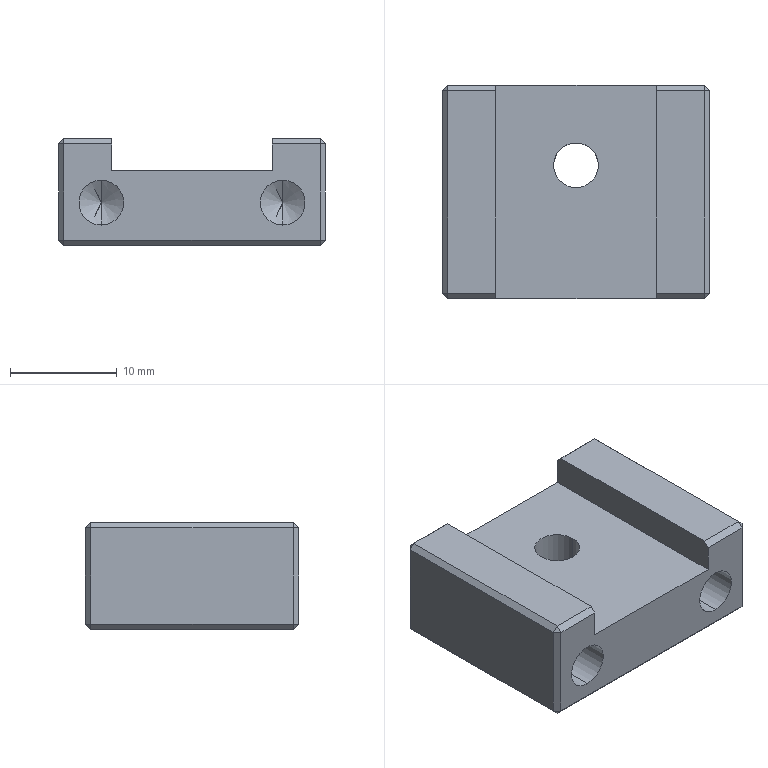Part | SolidWorks | features HoleWzd 2, Chamfer 1, Extrusion 1, ICE 1 | 1 solid | 42 faces | box 25 x 20 x 10 mm | volume 3625 mm3 | plane 32 | cylinder 6 | cone 4 | commonest cylinder face diameters 4.2 x6
STEP:
#1=CARTESIAN_POINT('',(-8.5,2.4,6.1));
#2=VERTEX_POINT('',#1);
#3=CARTESIAN_POINT('',(-8.5,2.4,1.9));
#4=VERTEX_POINT('',#3);
#5=CARTESIAN_POINT('',(-8.5,2.4,4.));
#6=DIRECTION('',(0.,-1.,0.));
#7=DIRECTION('',(0.,0.,-1.));
#8=AXIS2_PLACEMENT_3D('',#5,#6,#7);
#9=CIRCLE('',#8,2.1);
#10=EDGE_CURVE('',#2,#4,#9,.T.);
#11=ORIENTED_EDGE('',*,*,#10,.F.);
#12=CARTESIAN_POINT('',(-8.5,-10.,6.1));
#13=VERTEX_POINT('',#12);
#14=CARTESIAN_POINT('',(-8.5,-10.,6.1));
#15=DIRECTION('',(0.,-1.,0.));
#16=VECTOR('',#15,1000.);
#17=LINE('',#14,#16);
#18=EDGE_CURVE('',#2,#13,#17,.T.);
#19=ORIENTED_EDGE('',*,*,#18,.T.);
#20=CARTESIAN_POINT('',(-8.5,-10.,1.9));
#21=VERTEX_POINT('',#20);
#22=CARTESIAN_POINT('',(-8.5,-10.,4.));
#23=DIRECTION('',(0.,-1.,0.));
#24=DIRECTION('',(0.,0.,-1.));
#25=AXIS2_PLACEMENT_3D('',#22,#23,#24);
#26=CIRCLE('',#25,2.1);
#27=EDGE_CURVE('',#13,#21,#26,.T.);
#28=ORIENTED_EDGE('',*,*,#27,.T.);
#29=CARTESIAN_POINT('',(-8.5,-10.,1.9));
#30=DIRECTION('',(0.,-1.,0.));
#31=VECTOR('',#30,1000.);
#32=LINE('',#29,#31);
#33=EDGE_CURVE('',#4,#21,#32,.T.);
#34=ORIENTED_EDGE('',*,*,#33,.F.);
#35=EDGE_LOOP('',(#11,#19,#28,#34));
#36=FACE_OUTER_BOUND('',#35,.T.);
#37=CARTESIAN_POINT('',(-8.5,-10.,4.));
#38=DIRECTION('',(0.,-1.,0.));
#39=DIRECTION('',(0.,0.,-1.));
#40=AXIS2_PLACEMENT_3D('',#37,#38,#39);
#41=CYLINDRICAL_SURFACE('',#40,2.1);
#42=ADVANCED_FACE('',(#36),#41,.F.);
#43=CARTESIAN_POINT('',(-8.5,3.662,4.));
#44=VERTEX_POINT('',#43);
#45=CARTESIAN_POINT('',(-8.5,2.4,1.9));
#46=DIRECTION('',(0.,-0.515,-0.8572));
#47=VECTOR('',#46,1000.);
#48=LINE('',#45,#47);
#49=EDGE_CURVE('',#44,#4,#48,.T.);
#50=ORIENTED_EDGE('',*,*,#49,.F.);
#51=CARTESIAN_POINT('',(-8.5,2.4,6.1));
#52=DIRECTION('',(0.,-0.515,0.8572));
#53=VECTOR('',#52,1000.);
#54=LINE('',#51,#53);
#55=EDGE_CURVE('',#44,#2,#54,.T.);
#56=ORIENTED_EDGE('',*,*,#55,.T.);
#57=ORIENTED_EDGE('',*,*,#10,.T.);
#58=EDGE_LOOP('',(#50,#56,#57));
#59=FACE_OUTER_BOUND('',#58,.T.);
#60=CARTESIAN_POINT('',(-8.5,2.4,4.));
#61=DIRECTION('',(0.,-1.,0.));
#62=DIRECTION('',(0.,0.,-1.));
#63=AXIS2_PLACEMENT_3D('',#60,#61,#62);
#64=CONICAL_SURFACE('',#63,2.1,1.03);
#65=ADVANCED_FACE('',(#59),#64,.F.);
#66=CARTESIAN_POINT('',(8.5,2.4,6.1));
#67=VERTEX_POINT('',#66);
#68=CARTESIAN_POINT('',(8.5,2.4,1.9));
#69=VERTEX_POINT('',#68);
#70=CARTESIAN_POINT('',(8.5,2.4,4.));
#71=DIRECTION('',(0.,-1.,0.));
#72=DIRECTION('',(0.,0.,-1.));
#73=AXIS2_PLACEMENT_3D('',#70,#71,#72);
#74=CIRCLE('',#73,2.1);
#75=EDGE_CURVE('',#67,#69,#74,.T.);
#76=ORIENTED_EDGE('',*,*,#75,.F.);
#77=CARTESIAN_POINT('',(8.5,-10.,6.1));
#78=VERTEX_POINT('',#77);
#79=CARTESIAN_POINT('',(8.5,-10.,6.1));
#80=DIRECTION('',(0.,-1.,0.));
#81=VECTOR('',#80,1000.);
#82=LINE('',#79,#81);
#83=EDGE_CURVE('',#67,#78,#82,.T.);
#84=ORIENTED_EDGE('',*,*,#83,.T.);
#85=CARTESIAN_POINT('',(8.5,-10.,1.9));
#86=VERTEX_POINT('',#85);
#87=CARTESIAN_POINT('',(8.5,-10.,4.));
#88=DIRECTION('',(0.,-1.,0.));
#89=DIRECTION('',(0.,0.,-1.));
#90=AXIS2_PLACEMENT_3D('',#87,#88,#89);
#91=CIRCLE('',#90,2.1);
#92=EDGE_CURVE('',#78,#86,#91,.T.);
#93=ORIENTED_EDGE('',*,*,#92,.T.);
#94=CARTESIAN_POINT('',(8.5,-10.,1.9));
#95=DIRECTION('',(0.,-1.,0.));
#96=VECTOR('',#95,1000.);
#97=LINE('',#94,#96);
#98=EDGE_CURVE('',#69,#86,#97,.T.);
#99=ORIENTED_EDGE('',*,*,#98,.F.);
#100=EDGE_LOOP('',(#76,#84,#93,#99));
#101=FACE_OUTER_BOUND('',#100,.T.);
#102=CARTESIAN_POINT('',(8.5,-10.,4.));
#103=DIRECTION('',(0.,-1.,0.));
#104=DIRECTION('',(0.,0.,-1.));
#105=AXIS2_PLACEMENT_3D('',#102,#103,#104);
#106=CYLINDRICAL_SURFACE('',#105,2.1);
#107=ADVANCED_FACE('',(#101),#106,.F.);
#108=CARTESIAN_POINT('',(8.5,3.662,4.));
#109=VERTEX_POINT('',#108);
#110=CARTESIAN_POINT('',(8.5,2.4,1.9));
#111=DIRECTION('',(0.,-0.515,-0.8572));
#112=VECTOR('',#111,1000.);
#113=LINE('',#110,#112);
#114=EDGE_CURVE('',#109,#69,#113,.T.);
#115=ORIENTED_EDGE('',*,*,#114,.F.);
#116=CARTESIAN_POINT('',(8.5,2.4,6.1));
#117=DIRECTION('',(0.,-0.515,0.8572));
#118=VECTOR('',#117,1000.);
#119=LINE('',#116,#118);
#120=EDGE_CURVE('',#109,#67,#119,.T.);
#121=ORIENTED_EDGE('',*,*,#120,.T.);
#122=ORIENTED_EDGE('',*,*,#75,.T.);
#123=EDGE_LOOP('',(#115,#121,#122));
#124=FACE_OUTER_BOUND('',#123,.T.);
#125=CARTESIAN_POINT('',(8.5,2.4,4.));
#126=DIRECTION('',(0.,-1.,0.));
#127=DIRECTION('',(0.,0.,-1.));
#128=AXIS2_PLACEMENT_3D('',#125,#126,#127);
#129=CONICAL_SURFACE('',#128,2.1,1.03);
#130=ADVANCED_FACE('',(#124),#129,.F.);
#131=CARTESIAN_POINT('',(-2.1,2.5,0.));
#132=VERTEX_POINT('',#131);
#133=CARTESIAN_POINT('',(2.1,2.5,0.));
#134=VERTEX_POINT('',#133);
#135=CARTESIAN_POINT('',(0.,2.5,0.));
#136=DIRECTION('',(0.,0.,1.));
#137=DIRECTION('',(1.,0.,0.));
#138=AXIS2_PLACEMENT_3D('',#135,#136,#137);
#139=CIRCLE('',#138,2.1);
#140=EDGE_CURVE('',#132,#134,#139,.T.);
#141=ORIENTED_EDGE('',*,*,#140,.F.);
#142=CARTESIAN_POINT('',(-2.1,2.5,7.));
#143=VERTEX_POINT('',#142);
#144=CARTESIAN_POINT('',(-2.1,2.5,7.));
#145=DIRECTION('',(0.,0.,1.));
#146=VECTOR('',#145,1000.);
#147=LINE('',#144,#146);
#148=EDGE_CURVE('',#132,#143,#147,.T.);
#149=ORIENTED_EDGE('',*,*,#148,.T.);
#150=CARTESIAN_POINT('',(2.1,2.5,7.));
#151=VERTEX_POINT('',#150);
#152=CARTESIAN_POINT('',(0.,2.5,7.));
#153=DIRECTION('',(0.,0.,1.));
#154=DIRECTION('',(1.,0.,0.));
#155=AXIS2_PLACEMENT_3D('',#152,#153,#154);
#156=CIRCLE('',#155,2.1);
#157=EDGE_CURVE('',#143,#151,#156,.T.);
#158=ORIENTED_EDGE('',*,*,#157,.T.);
#159=CARTESIAN_POINT('',(2.1,2.5,7.));
#160=DIRECTION('',(0.,0.,1.));
#161=VECTOR('',#160,1000.);
#162=LINE('',#159,#161);
#163=EDGE_CURVE('',#134,#151,#162,.T.);
#164=ORIENTED_EDGE('',*,*,#163,.F.);
#165=EDGE_LOOP('',(#141,#149,#158,#164));
#166=FACE_OUTER_BOUND('',#165,.T.);
#167=CARTESIAN_POINT('',(0.,2.5,7.));
#168=DIRECTION('',(0.,0.,1.));
#169=DIRECTION('',(1.,0.,0.));
#170=AXIS2_PLACEMENT_3D('',#167,#168,#169);
#171=CYLINDRICAL_SURFACE('',#170,2.1);
#172=ADVANCED_FACE('',(#166),#171,.F.);
#173=CARTESIAN_POINT('',(12.,-10.,0.5));
#174=VERTEX_POINT('',#173);
#175=CARTESIAN_POINT('',(12.,-10.,9.5));
#176=VERTEX_POINT('',#175);
#177=CARTESIAN_POINT('',(12.,-10.,10.));
#178=DIRECTION('',(0.,0.,1.));
#179=VECTOR('',#178,1000.);
#180=LINE('',#177,#179);
#181=EDGE_CURVE('',#174,#176,#180,.T.);
#182=ORIENTED_EDGE('',*,*,#181,.T.);
#183=CARTESIAN_POINT('',(7.5,-10.,9.5));
#184=VERTEX_POINT('',#183);
#185=CARTESIAN_POINT('',(-12.5,-10.,9.5));
#186=DIRECTION('',(-1.,0.,0.));
#187=VECTOR('',#186,1000.);
#188=LINE('',#185,#187);
#189=EDGE_CURVE('',#176,#184,#188,.T.);
#190=ORIENTED_EDGE('',*,*,#189,.T.);
#191=CARTESIAN_POINT('',(7.5,-10.,7.));
#192=VERTEX_POINT('',#191);
#193=CARTESIAN_POINT('',(7.5,-10.,7.));
#194=DIRECTION('',(0.,0.,1.));
#195=VECTOR('',#194,1000.);
#196=LINE('',#193,#195);
#197=EDGE_CURVE('',#192,#184,#196,.T.);
#198=ORIENTED_EDGE('',*,*,#197,.F.);
#199=CARTESIAN_POINT('',(-7.5,-10.,7.));
#200=VERTEX_POINT('',#199);
#201=CARTESIAN_POINT('',(-7.5,-10.,7.));
#202=DIRECTION('',(1.,0.,0.));
#203=VECTOR('',#202,1000.);
#204=LINE('',#201,#203);
#205=EDGE_CURVE('',#200,#192,#204,.T.);
#206=ORIENTED_EDGE('',*,*,#205,.F.);
#207=CARTESIAN_POINT('',(-7.5,-10.,9.5));
#208=VERTEX_POINT('',#207);
#209=CARTESIAN_POINT('',(-7.5,-10.,7.));
#210=DIRECTION('',(0.,0.,1.));
#211=VECTOR('',#210,1000.);
#212=LINE('',#209,#211);
#213=EDGE_CURVE('',#200,#208,#212,.T.);
#214=ORIENTED_EDGE('',*,*,#213,.T.);
#215=CARTESIAN_POINT('',(-12.,-10.,9.5));
#216=VERTEX_POINT('',#215);
#217=CARTESIAN_POINT('',(-12.5,-10.,9.5));
#218=DIRECTION('',(-1.,0.,0.));
#219=VECTOR('',#218,1000.);
#220=LINE('',#217,#219);
#221=EDGE_CURVE('',#208,#216,#220,.T.);
#222=ORIENTED_EDGE('',*,*,#221,.T.);
#223=CARTESIAN_POINT('',(-12.,-10.,0.5));
#224=VERTEX_POINT('',#223);
#225=CARTESIAN_POINT('',(-12.,-10.,10.));
#226=DIRECTION('',(0.,0.,-1.));
#227=VECTOR('',#226,1000.);
#228=LINE('',#225,#227);
#229=EDGE_CURVE('',#216,#224,#228,.T.);
#230=ORIENTED_EDGE('',*,*,#229,.T.);
#231=CARTESIAN_POINT('',(12.5,-10.,0.5));
#232=DIRECTION('',(1.,0.,0.));
#233=VECTOR('',#232,1000.);
#234=LINE('',#231,#233);
#235=EDGE_CURVE('',#224,#174,#234,.T.);
#236=ORIENTED_EDGE('',*,*,#235,.T.);
#237=EDGE_LOOP('',(#182,#190,#198,#206,#214,#222,#230,#236));
#238=FACE_OUTER_BOUND('',#237,.T.);
#239=CARTESIAN_POINT('',(8.5,-10.,4.));
#240=DIRECTION('',(0.,-1.,0.));
#241=DIRECTION('',(0.,0.,-1.));
#242=AXIS2_PLACEMENT_3D('',#239,#240,#241);
#243=CIRCLE('',#242,2.1);
#244=EDGE_CURVE('',#86,#78,#243,.T.);
#245=ORIENTED_EDGE('',*,*,#244,.F.);
#246=ORIENTED_EDGE('',*,*,#92,.F.);
#247=EDGE_LOOP('',(#245,#246));
#248=FACE_BOUND('',#247,.T.);
#249=CARTESIAN_POINT('',(-8.5,-10.,4.));
#250=DIRECTION('',(0.,-1.,0.));
#251=DIRECTION('',(0.,0.,-1.));
#252=AXIS2_PLACEMENT_3D('',#249,#250,#251);
#253=CIRCLE('',#252,2.1);
#254=EDGE_CURVE('',#21,#13,#253,.T.);
#255=ORIENTED_EDGE('',*,*,#254,.F.);
#256=ORIENTED_EDGE('',*,*,#27,.F.);
#257=EDGE_LOOP('',(#255,#256));
#258=FACE_BOUND('',#257,.T.);
#259=CARTESIAN_POINT('',(-12.5,-10.,10.));
#260=DIRECTION('',(0.,1.,0.));
#261=DIRECTION('',(0.,0.,1.));
#262=AXIS2_PLACEMENT_3D('',#259,#260,#261);
#263=PLANE('',#262);
#264=ADVANCED_FACE('',(#238,#248,#258),#263,.F.);
#265=CARTESIAN_POINT('',(7.5,-9.5,10.));
#266=VERTEX_POINT('',#265);
#267=CARTESIAN_POINT('',(7.5,9.5,10.));
#268=VERTEX_POINT('',#267);
#269=CARTESIAN_POINT('',(7.5,10.,10.));
#270=DIRECTION('',(0.,1.,0.));
#271=VECTOR('',#270,1000.);
#272=LINE('',#269,#271);
#273=EDGE_CURVE('',#266,#268,#272,.T.);
#274=ORIENTED_EDGE('',*,*,#273,.F.);
#275=CARTESIAN_POINT('',(12.,-9.5,10.));
#276=VERTEX_POINT('',#275);
#277=CARTESIAN_POINT('',(0.,-9.5,10.));
#278=DIRECTION('',(1.,0.,0.));
#279=VECTOR('',#278,1000.);
#280=LINE('',#277,#279);
#281=EDGE_CURVE('',#266,#276,#280,.T.);
#282=ORIENTED_EDGE('',*,*,#281,.T.);
#283=CARTESIAN_POINT('',(12.,9.5,10.));
#284=VERTEX_POINT('',#283);
#285=CARTESIAN_POINT('',(12.,0.,10.));
#286=DIRECTION('',(0.,1.,0.));
#287=VECTOR('',#286,1000.);
#288=LINE('',#285,#287);
#289=EDGE_CURVE('',#276,#284,#288,.T.);
#290=ORIENTED_EDGE('',*,*,#289,.T.);
#291=CARTESIAN_POINT('',(0.,9.5,10.));
#292=DIRECTION('',(-1.,0.,0.));
#293=VECTOR('',#292,1000.);
#294=LINE('',#291,#293);
#295=EDGE_CURVE('',#284,#268,#294,.T.);
#296=ORIENTED_EDGE('',*,*,#295,.T.);
#297=EDGE_LOOP('',(#274,#282,#290,#296));
#298=FACE_OUTER_BOUND('',#297,.T.);
#299=CARTESIAN_POINT('',(0.,0.,10.));
#300=DIRECTION('',(0.,0.,-1.));
#301=DIRECTION('',(-1.,0.,0.));
#302=AXIS2_PLACEMENT_3D('',#299,#300,#301);
#303=PLANE('',#302);
#304=ADVANCED_FACE('',(#298),#303,.F.);
#305=CARTESIAN_POINT('',(12.5,9.5,0.5));
#306=VERTEX_POINT('',#305);
#307=CARTESIAN_POINT('',(12.5,9.5,9.5));
#308=VERTEX_POINT('',#307);
#309=CARTESIAN_POINT('',(12.5,9.5,10.));
#310=DIRECTION('',(0.,0.,1.));
#311=VECTOR('',#310,1000.);
#312=LINE('',#309,#311);
#313=EDGE_CURVE('',#306,#308,#312,.T.);
#314=ORIENTED_EDGE('',*,*,#313,.T.);
#315=CARTESIAN_POINT('',(12.5,-9.5,9.5));
#316=VERTEX_POINT('',#315);
#317=CARTESIAN_POINT('',(12.5,-10.,9.5));
#318=DIRECTION('',(0.,-1.,0.));
#319=VECTOR('',#318,1000.);
#320=LINE('',#317,#319);
#321=EDGE_CURVE('',#308,#316,#320,.T.);
#322=ORIENTED_EDGE('',*,*,#321,.T.);
#323=CARTESIAN_POINT('',(12.5,-9.5,0.5));
#324=VERTEX_POINT('',#323);
#325=CARTESIAN_POINT('',(12.5,-9.5,10.));
#326=DIRECTION('',(0.,0.,-1.));
#327=VECTOR('',#326,1000.);
#328=LINE('',#325,#327);
#329=EDGE_CURVE('',#316,#324,#328,.T.);
#330=ORIENTED_EDGE('',*,*,#329,.T.);
#331=CARTESIAN_POINT('',(12.5,10.,0.5));
#332=DIRECTION('',(0.,1.,0.));
#333=VECTOR('',#332,1000.);
#334=LINE('',#331,#333);
#335=EDGE_CURVE('',#324,#306,#334,.T.);
#336=ORIENTED_EDGE('',*,*,#335,.T.);
#337=EDGE_LOOP('',(#314,#322,#330,#336));
#338=FACE_OUTER_BOUND('',#337,.T.);
#339=CARTESIAN_POINT('',(12.5,-10.,10.));
#340=DIRECTION('',(-1.,0.,0.));
#341=DIRECTION('',(0.,0.,1.));
#342=AXIS2_PLACEMENT_3D('',#339,#340,#341);
#343=PLANE('',#342);
#344=ADVANCED_FACE('',(#338),#343,.F.);
#345=CARTESIAN_POINT('',(7.5,10.,7.));
#346=VERTEX_POINT('',#345);
#347=CARTESIAN_POINT('',(7.5,10.,9.5));
#348=VERTEX_POINT('',#347);
#349=CARTESIAN_POINT('',(7.5,10.,7.));
#350=DIRECTION('',(0.,0.,1.));
#351=VECTOR('',#350,1000.);
#352=LINE('',#349,#351);
#353=EDGE_CURVE('',#346,#348,#352,.T.);
#354=ORIENTED_EDGE('',*,*,#353,.T.);
#355=CARTESIAN_POINT('',(12.,10.,9.5));
#356=VERTEX_POINT('',#355);
#357=CARTESIAN_POINT('',(-12.5,10.,9.5));
#358=DIRECTION('',(1.,0.,0.));
#359=VECTOR('',#358,1000.);
#360=LINE('',#357,#359);
#361=EDGE_CURVE('',#348,#356,#360,.T.);
#362=ORIENTED_EDGE('',*,*,#361,.T.);
#363=CARTESIAN_POINT('',(12.,10.,0.5));
#364=VERTEX_POINT('',#363);
#365=CARTESIAN_POINT('',(12.,10.,10.));
#366=DIRECTION('',(0.,0.,-1.));
#367=VECTOR('',#366,1000.);
#368=LINE('',#365,#367);
#369=EDGE_CURVE('',#356,#364,#368,.T.);
#370=ORIENTED_EDGE('',*,*,#369,.T.);
#371=CARTESIAN_POINT('',(-12.,10.,0.5));
#372=VERTEX_POINT('',#371);
#373=CARTESIAN_POINT('',(-12.5,10.,0.5));
#374=DIRECTION('',(-1.,0.,0.));
#375=VECTOR('',#374,1000.);
#376=LINE('',#373,#375);
#377=EDGE_CURVE('',#364,#372,#376,.T.);
#378=ORIENTED_EDGE('',*,*,#377,.T.);
#379=CARTESIAN_POINT('',(-12.,10.,9.5));
#380=VERTEX_POINT('',#379);
#381=CARTESIAN_POINT('',(-12.,10.,10.));
#382=DIRECTION('',(0.,0.,1.));
#383=VECTOR('',#382,1000.);
#384=LINE('',#381,#383);
#385=EDGE_CURVE('',#372,#380,#384,.T.);
#386=ORIENTED_EDGE('',*,*,#385,.T.);
#387=CARTESIAN_POINT('',(-7.5,10.,9.5));
#388=VERTEX_POINT('',#387);
#389=CARTESIAN_POINT('',(-12.5,10.,9.5));
#390=DIRECTION('',(1.,0.,0.));
#391=VECTOR('',#390,1000.);
#392=LINE('',#389,#391);
#393=EDGE_CURVE('',#380,#388,#392,.T.);
#394=ORIENTED_EDGE('',*,*,#393,.T.);
#395=CARTESIAN_POINT('',(-7.5,10.,7.));
#396=VERTEX_POINT('',#395);
#397=CARTESIAN_POINT('',(-7.5,10.,7.));
#398=DIRECTION('',(0.,0.,1.));
#399=VECTOR('',#398,1000.);
#400=LINE('',#397,#399);
#401=EDGE_CURVE('',#396,#388,#400,.T.);
#402=ORIENTED_EDGE('',*,*,#401,.F.);
#403=CARTESIAN_POINT('',(-7.5,10.,7.));
#404=DIRECTION('',(-1.,0.,0.));
#405=VECTOR('',#404,1000.);
#406=LINE('',#403,#405);
#407=EDGE_CURVE('',#346,#396,#406,.T.);
#408=ORIENTED_EDGE('',*,*,#407,.F.);
#409=EDGE_LOOP('',(#354,#362,#370,#378,#386,#394,#402,#408));
#410=FACE_OUTER_BOUND('',#409,.T.);
#411=CARTESIAN_POINT('',(-12.5,10.,10.));
#412=DIRECTION('',(0.,-1.,0.));
#413=DIRECTION('',(0.,0.,-1.));
#414=AXIS2_PLACEMENT_3D('',#411,#412,#413);
#415=PLANE('',#414);
#416=ADVANCED_FACE('',(#410),#415,.F.);
#417=CARTESIAN_POINT('',(-12.5,9.5,0.5));
#418=VERTEX_POINT('',#417);
#419=CARTESIAN_POINT('',(-12.5,-9.5,0.5));
#420=VERTEX_POINT('',#419);
#421=CARTESIAN_POINT('',(-12.5,-10.,0.5));
#422=DIRECTION('',(0.,-1.,0.));
#423=VECTOR('',#422,1000.);
#424=LINE('',#421,#423);
#425=EDGE_CURVE('',#418,#420,#424,.T.);
#426=ORIENTED_EDGE('',*,*,#425,.T.);
#427=CARTESIAN_POINT('',(-12.5,-9.5,9.5));
#428=VERTEX_POINT('',#427);
#429=CARTESIAN_POINT('',(-12.5,-9.5,10.));
#430=DIRECTION('',(0.,0.,1.));
#431=VECTOR('',#430,1000.);
#432=LINE('',#429,#431);
#433=EDGE_CURVE('',#420,#428,#432,.T.);
#434=ORIENTED_EDGE('',*,*,#433,.T.);
#435=CARTESIAN_POINT('',(-12.5,9.5,9.5));
#436=VERTEX_POINT('',#435);
#437=CARTESIAN_POINT('',(-12.5,-10.,9.5));
#438=DIRECTION('',(0.,1.,0.));
#439=VECTOR('',#438,1000.);
#440=LINE('',#437,#439);
#441=EDGE_CURVE('',#428,#436,#440,.T.);
#442=ORIENTED_EDGE('',*,*,#441,.T.);
#443=CARTESIAN_POINT('',(-12.5,9.5,10.));
#444=DIRECTION('',(0.,0.,-1.));
#445=VECTOR('',#444,1000.);
#446=LINE('',#443,#445);
#447=EDGE_CURVE('',#436,#418,#446,.T.);
#448=ORIENTED_EDGE('',*,*,#447,.T.);
#449=EDGE_LOOP('',(#426,#434,#442,#448));
#450=FACE_OUTER_BOUND('',#449,.T.);
#451=CARTESIAN_POINT('',(-12.5,-10.,10.));
#452=DIRECTION('',(1.,0.,0.));
#453=DIRECTION('',(0.,0.,-1.));
#454=AXIS2_PLACEMENT_3D('',#451,#452,#453);
#455=PLANE('',#454);
#456=ADVANCED_FACE('',(#450),#455,.F.);
#457=CARTESIAN_POINT('',(-12.,9.5,10.));
#458=VERTEX_POINT('',#457);
#459=CARTESIAN_POINT('',(-12.,-9.5,10.));
#460=VERTEX_POINT('',#459);
#461=CARTESIAN_POINT('',(-12.,0.,10.));
#462=DIRECTION('',(0.,-1.,0.));
#463=VECTOR('',#462,1000.);
#464=LINE('',#461,#463);
#465=EDGE_CURVE('',#458,#460,#464,.T.);
#466=ORIENTED_EDGE('',*,*,#465,.T.);
#467=CARTESIAN_POINT('',(-7.5,-9.5,10.));
#468=VERTEX_POINT('',#467);
#469=CARTESIAN_POINT('',(0.,-9.5,10.));
#470=DIRECTION('',(1.,0.,0.));
#471=VECTOR('',#470,1000.);
#472=LINE('',#469,#471);
#473=EDGE_CURVE('',#460,#468,#472,.T.);
#474=ORIENTED_EDGE('',*,*,#473,.T.);
#475=CARTESIAN_POINT('',(-7.5,9.5,10.));
#476=VERTEX_POINT('',#475);
#477=CARTESIAN_POINT('',(-7.5,10.,10.));
#478=DIRECTION('',(0.,-1.,0.));
#479=VECTOR('',#478,1000.);
#480=LINE('',#477,#479);
#481=EDGE_CURVE('',#476,#468,#480,.T.);
#482=ORIENTED_EDGE('',*,*,#481,.F.);
#483=CARTESIAN_POINT('',(0.,9.5,10.));
#484=DIRECTION('',(-1.,0.,0.));
#485=VECTOR('',#484,1000.);
#486=LINE('',#483,#485);
#487=EDGE_CURVE('',#476,#458,#486,.T.);
#488=ORIENTED_EDGE('',*,*,#487,.T.);
#489=EDGE_LOOP('',(#466,#474,#482,#488));
#490=FACE_OUTER_BOUND('',#489,.T.);
#491=CARTESIAN_POINT('',(0.,0.,10.));
#492=DIRECTION('',(0.,0.,-1.));
#493=DIRECTION('',(-1.,0.,0.));
#494=AXIS2_PLACEMENT_3D('',#491,#492,#493);
#495=PLANE('',#494);
#496=ADVANCED_FACE('',(#490),#495,.F.);
#497=CARTESIAN_POINT('',(-12.,9.5,0.));
#498=VERTEX_POINT('',#497);
#499=CARTESIAN_POINT('',(12.,9.5,0.));
#500=VERTEX_POINT('',#499);
#501=CARTESIAN_POINT('',(12.5,9.5,0.));
#502=DIRECTION('',(1.,0.,0.));
#503=VECTOR('',#502,1000.);
#504=LINE('',#501,#503);
#505=EDGE_CURVE('',#498,#500,#504,.T.);
#506=ORIENTED_EDGE('',*,*,#505,.T.);
#507=CARTESIAN_POINT('',(12.,-9.5,0.));
#508=VERTEX_POINT('',#507);
#509=CARTESIAN_POINT('',(12.,-10.,0.));
#510=DIRECTION('',(0.,-1.,0.));
#511=VECTOR('',#510,1000.);
#512=LINE('',#509,#511);
#513=EDGE_CURVE('',#500,#508,#512,.T.);
#514=ORIENTED_EDGE('',*,*,#513,.T.);
#515=CARTESIAN_POINT('',(-12.,-9.5,0.));
#516=VERTEX_POINT('',#515);
#517=CARTESIAN_POINT('',(-12.5,-9.5,0.));
#518=DIRECTION('',(-1.,0.,0.));
#519=VECTOR('',#518,1000.);
#520=LINE('',#517,#519);
#521=EDGE_CURVE('',#508,#516,#520,.T.);
#522=ORIENTED_EDGE('',*,*,#521,.T.);
#523=CARTESIAN_POINT('',(-12.,10.,0.));
#524=DIRECTION('',(0.,1.,0.));
#525=VECTOR('',#524,1000.);
#526=LINE('',#523,#525);
#527=EDGE_CURVE('',#516,#498,#526,.T.);
#528=ORIENTED_EDGE('',*,*,#527,.T.);
#529=EDGE_LOOP('',(#506,#514,#522,#528));
#530=FACE_OUTER_BOUND('',#529,.T.);
#531=CARTESIAN_POINT('',(0.,2.5,0.));
#532=DIRECTION('',(0.,0.,1.));
#533=DIRECTION('',(1.,0.,0.));
#534=AXIS2_PLACEMENT_3D('',#531,#532,#533);
#535=CIRCLE('',#534,2.1);
#536=EDGE_CURVE('',#134,#132,#535,.T.);
#537=ORIENTED_EDGE('',*,*,#536,.T.);
#538=ORIENTED_EDGE('',*,*,#140,.T.);
#539=EDGE_LOOP('',(#537,#538));
#540=FACE_BOUND('',#539,.T.);
#541=CARTESIAN_POINT('',(0.,0.,0.));
#542=DIRECTION('',(0.,0.,-1.));
#543=DIRECTION('',(-1.,0.,0.));
#544=AXIS2_PLACEMENT_3D('',#541,#542,#543);
#545=PLANE('',#544);
#546=ADVANCED_FACE('',(#530,#540),#545,.T.);
#547=ORIENTED_EDGE('',*,*,#197,.T.);
#548=CARTESIAN_POINT('',(7.5,-9.5,10.));
#549=DIRECTION('',(0.,0.7071,0.7071));
#550=VECTOR('',#549,1000.);
#551=LINE('',#548,#550);
#552=EDGE_CURVE('',#184,#266,#551,.T.);
#553=ORIENTED_EDGE('',*,*,#552,.T.);
#554=ORIENTED_EDGE('',*,*,#273,.T.);
#555=CARTESIAN_POINT('',(7.5,9.5,10.));
#556=DIRECTION('',(0.,0.7071,-0.7071));
#557=VECTOR('',#556,1000.);
#558=LINE('',#555,#557);
#559=EDGE_CURVE('',#268,#348,#558,.T.);
#560=ORIENTED_EDGE('',*,*,#559,.T.);
#561=ORIENTED_EDGE('',*,*,#353,.F.);
#562=CARTESIAN_POINT('',(7.5,10.,7.));
#563=DIRECTION('',(0.,1.,0.));
#564=VECTOR('',#563,1000.);
#565=LINE('',#562,#564);
#566=EDGE_CURVE('',#192,#346,#565,.T.);
#567=ORIENTED_EDGE('',*,*,#566,.F.);
#568=EDGE_LOOP('',(#547,#553,#554,#560,#561,#567));
#569=FACE_OUTER_BOUND('',#568,.T.);
#570=CARTESIAN_POINT('',(7.5,10.,7.));
#571=DIRECTION('',(1.,0.,0.));
#572=DIRECTION('',(0.,0.,-1.));
#573=AXIS2_PLACEMENT_3D('',#570,#571,#572);
#574=PLANE('',#573);
#575=ADVANCED_FACE('',(#569),#574,.F.);
#576=ORIENTED_EDGE('',*,*,#481,.T.);
#577=CARTESIAN_POINT('',(-7.5,-9.5,10.));
#578=DIRECTION('',(0.,-0.7071,-0.7071));
#579=VECTOR('',#578,1000.);
#580=LINE('',#577,#579);
#581=EDGE_CURVE('',#468,#208,#580,.T.);
#582=ORIENTED_EDGE('',*,*,#581,.T.);
#583=ORIENTED_EDGE('',*,*,#213,.F.);
#584=CARTESIAN_POINT('',(-7.5,10.,7.));
#585=DIRECTION('',(0.,-1.,0.));
#586=VECTOR('',#585,1000.);
#587=LINE('',#584,#586);
#588=EDGE_CURVE('',#396,#200,#587,.T.);
#589=ORIENTED_EDGE('',*,*,#588,.F.);
#590=ORIENTED_EDGE('',*,*,#401,.T.);
#591=CARTESIAN_POINT('',(-7.5,9.5,10.));
#592=DIRECTION('',(0.,-0.7071,0.7071));
#593=VECTOR('',#592,1000.);
#594=LINE('',#591,#593);
#595=EDGE_CURVE('',#388,#476,#594,.T.);
#596=ORIENTED_EDGE('',*,*,#595,.T.);
#597=EDGE_LOOP('',(#576,#582,#583,#589,#590,#596));
#598=FACE_OUTER_BOUND('',#597,.T.);
#599=CARTESIAN_POINT('',(-7.5,10.,7.));
#600=DIRECTION('',(-1.,0.,0.));
#601=DIRECTION('',(0.,0.,1.));
#602=AXIS2_PLACEMENT_3D('',#599,#600,#601);
#603=PLANE('',#602);
#604=ADVANCED_FACE('',(#598),#603,.F.);
#605=CARTESIAN_POINT('',(0.,2.5,7.));
#606=DIRECTION('',(0.,0.,1.));
#607=DIRECTION('',(1.,0.,0.));
#608=AXIS2_PLACEMENT_3D('',#605,#606,#607);
#609=CIRCLE('',#608,2.1);
#610=EDGE_CURVE('',#151,#143,#609,.T.);
#611=ORIENTED_EDGE('',*,*,#610,.F.);
#612=ORIENTED_EDGE('',*,*,#157,.F.);
#613=EDGE_LOOP('',(#611,#612));
#614=FACE_BOUND('',#613,.T.);
#615=ORIENTED_EDGE('',*,*,#566,.T.);
#616=ORIENTED_EDGE('',*,*,#407,.T.);
#617=ORIENTED_EDGE('',*,*,#588,.T.);
#618=ORIENTED_EDGE('',*,*,#205,.T.);
#619=EDGE_LOOP('',(#615,#616,#617,#618));
#620=FACE_OUTER_BOUND('',#619,.T.);
#621=CARTESIAN_POINT('',(0.,0.,7.));
#622=DIRECTION('',(0.,0.,1.));
#623=DIRECTION('',(1.,0.,0.));
#624=AXIS2_PLACEMENT_3D('',#621,#622,#623);
#625=PLANE('',#624);
#626=ADVANCED_FACE('',(#614,#620),#625,.T.);
#627=ORIENTED_EDGE('',*,*,#148,.F.);
#628=ORIENTED_EDGE('',*,*,#536,.F.);
#629=ORIENTED_EDGE('',*,*,#163,.T.);
#630=ORIENTED_EDGE('',*,*,#610,.T.);
#631=EDGE_LOOP('',(#627,#628,#629,#630));
#632=FACE_OUTER_BOUND('',#631,.T.);
#633=CARTESIAN_POINT('',(0.,2.5,7.));
#634=DIRECTION('',(0.,0.,1.));
#635=DIRECTION('',(1.,0.,0.));
#636=AXIS2_PLACEMENT_3D('',#633,#634,#635);
#637=CYLINDRICAL_SURFACE('',#636,2.1);
#638=ADVANCED_FACE('',(#632),#637,.F.);
#639=ORIENTED_EDGE('',*,*,#120,.F.);
#640=ORIENTED_EDGE('',*,*,#114,.T.);
#641=CARTESIAN_POINT('',(8.5,2.4,4.));
#642=DIRECTION('',(0.,-1.,0.));
#643=DIRECTION('',(0.,0.,-1.));
#644=AXIS2_PLACEMENT_3D('',#641,#642,#643);
#645=CIRCLE('',#644,2.1);
#646=EDGE_CURVE('',#69,#67,#645,.T.);
#647=ORIENTED_EDGE('',*,*,#646,.T.);
#648=EDGE_LOOP('',(#639,#640,#647));
#649=FACE_OUTER_BOUND('',#648,.T.);
#650=CARTESIAN_POINT('',(8.5,2.4,4.));
#651=DIRECTION('',(0.,-1.,0.));
#652=DIRECTION('',(0.,0.,-1.));
#653=AXIS2_PLACEMENT_3D('',#650,#651,#652);
#654=CONICAL_SURFACE('',#653,2.1,1.03);
#655=ADVANCED_FACE('',(#649),#654,.F.);
#656=ORIENTED_EDGE('',*,*,#83,.F.);
#657=ORIENTED_EDGE('',*,*,#646,.F.);
#658=ORIENTED_EDGE('',*,*,#98,.T.);
#659=ORIENTED_EDGE('',*,*,#244,.T.);
#660=EDGE_LOOP('',(#656,#657,#658,#659));
#661=FACE_OUTER_BOUND('',#660,.T.);
#662=CARTESIAN_POINT('',(8.5,-10.,4.));
#663=DIRECTION('',(0.,-1.,0.));
#664=DIRECTION('',(0.,0.,-1.));
#665=AXIS2_PLACEMENT_3D('',#662,#663,#664);
#666=CYLINDRICAL_SURFACE('',#665,2.1);
#667=ADVANCED_FACE('',(#661),#666,.F.);
#668=ORIENTED_EDGE('',*,*,#55,.F.);
#669=ORIENTED_EDGE('',*,*,#49,.T.);
#670=CARTESIAN_POINT('',(-8.5,2.4,4.));
#671=DIRECTION('',(0.,-1.,0.));
#672=DIRECTION('',(0.,0.,-1.));
#673=AXIS2_PLACEMENT_3D('',#670,#671,#672);
#674=CIRCLE('',#673,2.1);
#675=EDGE_CURVE('',#4,#2,#674,.T.);
#676=ORIENTED_EDGE('',*,*,#675,.T.);
#677=EDGE_LOOP('',(#668,#669,#676));
#678=FACE_OUTER_BOUND('',#677,.T.);
#679=CARTESIAN_POINT('',(-8.5,2.4,4.));
#680=DIRECTION('',(0.,-1.,0.));
#681=DIRECTION('',(0.,0.,-1.));
#682=AXIS2_PLACEMENT_3D('',#679,#680,#681);
#683=CONICAL_SURFACE('',#682,2.1,1.03);
#684=ADVANCED_FACE('',(#678),#683,.F.);
#685=ORIENTED_EDGE('',*,*,#18,.F.);
#686=ORIENTED_EDGE('',*,*,#675,.F.);
#687=ORIENTED_EDGE('',*,*,#33,.T.);
#688=ORIENTED_EDGE('',*,*,#254,.T.);
#689=EDGE_LOOP('',(#685,#686,#687,#688));
#690=FACE_OUTER_BOUND('',#689,.T.);
#691=CARTESIAN_POINT('',(-8.5,-10.,4.));
#692=DIRECTION('',(0.,-1.,0.));
#693=DIRECTION('',(0.,0.,-1.));
#694=AXIS2_PLACEMENT_3D('',#691,#692,#693);
#695=CYLINDRICAL_SURFACE('',#694,2.1);
#696=ADVANCED_FACE('',(#690),#695,.F.);
#697=CARTESIAN_POINT('',(-12.,9.5,10.));
#698=DIRECTION('',(0.,0.7071,-0.7071));
#699=VECTOR('',#698,1000.);
#700=LINE('',#697,#699);
#701=EDGE_CURVE('',#458,#380,#700,.T.);
#702=ORIENTED_EDGE('',*,*,#701,.F.);
#703=ORIENTED_EDGE('',*,*,#487,.F.);
#704=ORIENTED_EDGE('',*,*,#595,.F.);
#705=ORIENTED_EDGE('',*,*,#393,.F.);
#706=EDGE_LOOP('',(#702,#703,#704,#705));
#707=FACE_OUTER_BOUND('',#706,.T.);
#708=CARTESIAN_POINT('',(0.,9.5,10.));
#709=DIRECTION('',(0.,-0.7071,-0.7071));
#710=DIRECTION('',(-1.,0.,0.));
#711=AXIS2_PLACEMENT_3D('',#708,#709,#710);
#712=PLANE('',#711);
#713=ADVANCED_FACE('',(#707),#712,.F.);
#714=CARTESIAN_POINT('',(-12.,9.5,10.));
#715=DIRECTION('',(-0.7071,0.,-0.7071));
#716=VECTOR('',#715,1000.);
#717=LINE('',#714,#716);
#718=EDGE_CURVE('',#458,#436,#717,.T.);
#719=ORIENTED_EDGE('',*,*,#718,.F.);
#720=ORIENTED_EDGE('',*,*,#701,.T.);
#721=CARTESIAN_POINT('',(-12.25,9.75,9.5));
#722=DIRECTION('',(0.7071,0.7071,0.));
#723=VECTOR('',#722,1000.);
#724=LINE('',#721,#723);
#725=EDGE_CURVE('',#436,#380,#724,.T.);
#726=ORIENTED_EDGE('',*,*,#725,.F.);
#727=EDGE_LOOP('',(#719,#720,#726));
#728=FACE_OUTER_BOUND('',#727,.T.);
#729=CARTESIAN_POINT('',(-12.,9.5,10.));
#730=DIRECTION('',(-0.5774,0.5774,0.5774));
#731=DIRECTION('',(0.7071,0.,0.7071));
#732=AXIS2_PLACEMENT_3D('',#729,#730,#731);
#733=PLANE('',#732);
#734=ADVANCED_FACE('',(#728),#733,.T.);
#735=ORIENTED_EDGE('',*,*,#725,.T.);
#736=ORIENTED_EDGE('',*,*,#385,.F.);
#737=CARTESIAN_POINT('',(-12.,10.,0.5));
#738=DIRECTION('',(0.7071,0.7071,0.));
#739=VECTOR('',#738,1000.);
#740=LINE('',#737,#739);
#741=EDGE_CURVE('',#418,#372,#740,.T.);
#742=ORIENTED_EDGE('',*,*,#741,.F.);
#743=ORIENTED_EDGE('',*,*,#447,.F.);
#744=EDGE_LOOP('',(#735,#736,#742,#743));
#745=FACE_OUTER_BOUND('',#744,.T.);
#746=CARTESIAN_POINT('',(-12.5,9.5,10.));
#747=DIRECTION('',(0.7071,-0.7071,0.));
#748=DIRECTION('',(0.,0.,-1.));
#749=AXIS2_PLACEMENT_3D('',#746,#747,#748);
#750=PLANE('',#749);
#751=ADVANCED_FACE('',(#745),#750,.F.);
#752=ORIENTED_EDGE('',*,*,#718,.T.);
#753=ORIENTED_EDGE('',*,*,#441,.F.);
#754=CARTESIAN_POINT('',(-12.25,-9.5,9.75));
#755=DIRECTION('',(-0.7071,0.,-0.7071));
#756=VECTOR('',#755,1000.);
#757=LINE('',#754,#756);
#758=EDGE_CURVE('',#460,#428,#757,.T.);
#759=ORIENTED_EDGE('',*,*,#758,.F.);
#760=ORIENTED_EDGE('',*,*,#465,.F.);
#761=EDGE_LOOP('',(#752,#753,#759,#760));
#762=FACE_OUTER_BOUND('',#761,.T.);
#763=CARTESIAN_POINT('',(-12.,0.,10.));
#764=DIRECTION('',(0.7071,0.,-0.7071));
#765=DIRECTION('',(0.,-1.,0.));
#766=AXIS2_PLACEMENT_3D('',#763,#764,#765);
#767=PLANE('',#766);
#768=ADVANCED_FACE('',(#762),#767,.F.);
#769=ORIENTED_EDGE('',*,*,#581,.F.);
#770=ORIENTED_EDGE('',*,*,#473,.F.);
#771=CARTESIAN_POINT('',(-12.,-10.,9.5));
#772=DIRECTION('',(0.,0.7071,0.7071));
#773=VECTOR('',#772,1000.);
#774=LINE('',#771,#773);
#775=EDGE_CURVE('',#216,#460,#774,.T.);
#776=ORIENTED_EDGE('',*,*,#775,.F.);
#777=ORIENTED_EDGE('',*,*,#221,.F.);
#778=EDGE_LOOP('',(#769,#770,#776,#777));
#779=FACE_OUTER_BOUND('',#778,.T.);
#780=CARTESIAN_POINT('',(0.,-9.5,10.));
#781=DIRECTION('',(0.,0.7071,-0.7071));
#782=DIRECTION('',(1.,0.,0.));
#783=AXIS2_PLACEMENT_3D('',#780,#781,#782);
#784=PLANE('',#783);
#785=ADVANCED_FACE('',(#779),#784,.F.);
#786=CARTESIAN_POINT('',(-12.25,9.5,0.25));
#787=DIRECTION('',(0.7071,0.,-0.7071));
#788=VECTOR('',#787,1000.);
#789=LINE('',#786,#788);
#790=EDGE_CURVE('',#418,#498,#789,.T.);
#791=ORIENTED_EDGE('',*,*,#790,.F.);
#792=ORIENTED_EDGE('',*,*,#741,.T.);
#793=CARTESIAN_POINT('',(-12.,10.,0.5));
#794=DIRECTION('',(0.,0.7071,0.7071));
#795=VECTOR('',#794,1000.);
#796=LINE('',#793,#795);
#797=EDGE_CURVE('',#498,#372,#796,.T.);
#798=ORIENTED_EDGE('',*,*,#797,.F.);
#799=EDGE_LOOP('',(#791,#792,#798));
#800=FACE_OUTER_BOUND('',#799,.T.);
#801=CARTESIAN_POINT('',(-12.,10.,0.5));
#802=DIRECTION('',(-0.5774,0.5774,-0.5774));
#803=DIRECTION('',(-0.7071,0.,0.7071));
#804=AXIS2_PLACEMENT_3D('',#801,#802,#803);
#805=PLANE('',#804);
#806=ADVANCED_FACE('',(#800),#805,.T.);
#807=ORIENTED_EDGE('',*,*,#775,.T.);
#808=ORIENTED_EDGE('',*,*,#758,.T.);
#809=CARTESIAN_POINT('',(-12.,-10.,9.5));
#810=DIRECTION('',(-0.7071,0.7071,0.));
#811=VECTOR('',#810,1000.);
#812=LINE('',#809,#811);
#813=EDGE_CURVE('',#216,#428,#812,.T.);
#814=ORIENTED_EDGE('',*,*,#813,.F.);
#815=EDGE_LOOP('',(#807,#808,#814));
#816=FACE_OUTER_BOUND('',#815,.T.);
#817=CARTESIAN_POINT('',(-12.,-10.,9.5));
#818=DIRECTION('',(-0.5774,-0.5774,0.5774));
#819=DIRECTION('',(0.7071,0.,0.7071));
#820=AXIS2_PLACEMENT_3D('',#817,#818,#819);
#821=PLANE('',#820);
#822=ADVANCED_FACE('',(#816),#821,.T.);
#823=ORIENTED_EDGE('',*,*,#797,.T.);
#824=ORIENTED_EDGE('',*,*,#377,.F.);
#825=CARTESIAN_POINT('',(12.,10.,0.5));
#826=DIRECTION('',(0.,0.7071,0.7071));
#827=VECTOR('',#826,1000.);
#828=LINE('',#825,#827);
#829=EDGE_CURVE('',#500,#364,#828,.T.);
#830=ORIENTED_EDGE('',*,*,#829,.F.);
#831=ORIENTED_EDGE('',*,*,#505,.F.);
#832=EDGE_LOOP('',(#823,#824,#830,#831));
#833=FACE_OUTER_BOUND('',#832,.T.);
#834=CARTESIAN_POINT('',(-12.5,10.,0.5));
#835=DIRECTION('',(0.,0.7071,-0.7071));
#836=DIRECTION('',(1.,0.,0.));
#837=AXIS2_PLACEMENT_3D('',#834,#835,#836);
#838=PLANE('',#837);
#839=ADVANCED_FACE('',(#833),#838,.T.);
#840=ORIENTED_EDGE('',*,*,#790,.T.);
#841=ORIENTED_EDGE('',*,*,#527,.F.);
#842=CARTESIAN_POINT('',(-12.,-9.5,0.));
#843=DIRECTION('',(0.7071,0.,-0.7071));
#844=VECTOR('',#843,1000.);
#845=LINE('',#842,#844);
#846=EDGE_CURVE('',#420,#516,#845,.T.);
#847=ORIENTED_EDGE('',*,*,#846,.F.);
#848=ORIENTED_EDGE('',*,*,#425,.F.);
#849=EDGE_LOOP('',(#840,#841,#847,#848));
#850=FACE_OUTER_BOUND('',#849,.T.);
#851=CARTESIAN_POINT('',(-12.5,-10.,0.5));
#852=DIRECTION('',(-0.7071,0.,-0.7071));
#853=DIRECTION('',(0.,1.,0.));
#854=AXIS2_PLACEMENT_3D('',#851,#852,#853);
#855=PLANE('',#854);
#856=ADVANCED_FACE('',(#850),#855,.T.);
#857=ORIENTED_EDGE('',*,*,#813,.T.);
#858=ORIENTED_EDGE('',*,*,#433,.F.);
#859=CARTESIAN_POINT('',(-12.25,-9.75,0.5));
#860=DIRECTION('',(-0.7071,0.7071,0.));
#861=VECTOR('',#860,1000.);
#862=LINE('',#859,#861);
#863=EDGE_CURVE('',#224,#420,#862,.T.);
#864=ORIENTED_EDGE('',*,*,#863,.F.);
#865=ORIENTED_EDGE('',*,*,#229,.F.);
#866=EDGE_LOOP('',(#857,#858,#864,#865));
#867=FACE_OUTER_BOUND('',#866,.T.);
#868=CARTESIAN_POINT('',(-12.,-10.,10.));
#869=DIRECTION('',(0.7071,0.7071,0.));
#870=DIRECTION('',(0.,0.,-1.));
#871=AXIS2_PLACEMENT_3D('',#868,#869,#870);
#872=PLANE('',#871);
#873=ADVANCED_FACE('',(#867),#872,.F.);
#874=CARTESIAN_POINT('',(12.25,9.5,0.25));
#875=DIRECTION('',(0.7071,0.,0.7071));
#876=VECTOR('',#875,1000.);
#877=LINE('',#874,#876);
#878=EDGE_CURVE('',#500,#306,#877,.T.);
#879=ORIENTED_EDGE('',*,*,#878,.F.);
#880=ORIENTED_EDGE('',*,*,#829,.T.);
#881=CARTESIAN_POINT('',(12.,10.,0.5));
#882=DIRECTION('',(-0.7071,0.7071,0.));
#883=VECTOR('',#882,1000.);
#884=LINE('',#881,#883);
#885=EDGE_CURVE('',#306,#364,#884,.T.);
#886=ORIENTED_EDGE('',*,*,#885,.F.);
#887=EDGE_LOOP('',(#879,#880,#886));
#888=FACE_OUTER_BOUND('',#887,.T.);
#889=CARTESIAN_POINT('',(12.,10.,0.5));
#890=DIRECTION('',(0.5774,0.5774,-0.5774));
#891=DIRECTION('',(-0.7071,0.,-0.7071));
#892=AXIS2_PLACEMENT_3D('',#889,#890,#891);
#893=PLANE('',#892);
#894=ADVANCED_FACE('',(#888),#893,.T.);
#895=ORIENTED_EDGE('',*,*,#863,.T.);
#896=ORIENTED_EDGE('',*,*,#846,.T.);
#897=CARTESIAN_POINT('',(-12.,-9.5,0.));
#898=DIRECTION('',(0.,0.7071,-0.7071));
#899=VECTOR('',#898,1000.);
#900=LINE('',#897,#899);
#901=EDGE_CURVE('',#224,#516,#900,.T.);
#902=ORIENTED_EDGE('',*,*,#901,.F.);
#903=EDGE_LOOP('',(#895,#896,#902));
#904=FACE_OUTER_BOUND('',#903,.T.);
#905=CARTESIAN_POINT('',(-12.,-9.5,0.));
#906=DIRECTION('',(-0.5774,-0.5774,-0.5774));
#907=DIRECTION('',(-0.7071,0.,0.7071));
#908=AXIS2_PLACEMENT_3D('',#905,#906,#907);
#909=PLANE('',#908);
#910=ADVANCED_FACE('',(#904),#909,.T.);
#911=ORIENTED_EDGE('',*,*,#559,.F.);
#912=ORIENTED_EDGE('',*,*,#295,.F.);
#913=CARTESIAN_POINT('',(12.,10.,9.5));
#914=DIRECTION('',(0.,-0.7071,0.7071));
#915=VECTOR('',#914,1000.);
#916=LINE('',#913,#915);
#917=EDGE_CURVE('',#356,#284,#916,.T.);
#918=ORIENTED_EDGE('',*,*,#917,.F.);
#919=ORIENTED_EDGE('',*,*,#361,.F.);
#920=EDGE_LOOP('',(#911,#912,#918,#919));
#921=FACE_OUTER_BOUND('',#920,.T.);
#922=CARTESIAN_POINT('',(0.,9.5,10.));
#923=DIRECTION('',(0.,-0.7071,-0.7071));
#924=DIRECTION('',(-1.,0.,0.));
#925=AXIS2_PLACEMENT_3D('',#922,#923,#924);
#926=PLANE('',#925);
#927=ADVANCED_FACE('',(#921),#926,.F.);
#928=ORIENTED_EDGE('',*,*,#885,.T.);
#929=ORIENTED_EDGE('',*,*,#369,.F.);
#930=CARTESIAN_POINT('',(12.,10.,9.5));
#931=DIRECTION('',(-0.7071,0.7071,0.));
#932=VECTOR('',#931,1000.);
#933=LINE('',#930,#932);
#934=EDGE_CURVE('',#308,#356,#933,.T.);
#935=ORIENTED_EDGE('',*,*,#934,.F.);
#936=ORIENTED_EDGE('',*,*,#313,.F.);
#937=EDGE_LOOP('',(#928,#929,#935,#936));
#938=FACE_OUTER_BOUND('',#937,.T.);
#939=CARTESIAN_POINT('',(12.,10.,10.));
#940=DIRECTION('',(-0.7071,-0.7071,0.));
#941=DIRECTION('',(0.,0.,-1.));
#942=AXIS2_PLACEMENT_3D('',#939,#940,#941);
#943=PLANE('',#942);
#944=ADVANCED_FACE('',(#938),#943,.F.);
#945=ORIENTED_EDGE('',*,*,#878,.T.);
#946=ORIENTED_EDGE('',*,*,#335,.F.);
#947=CARTESIAN_POINT('',(12.5,-9.5,0.5));
#948=DIRECTION('',(0.7071,0.,0.7071));
#949=VECTOR('',#948,1000.);
#950=LINE('',#947,#949);
#951=EDGE_CURVE('',#508,#324,#950,.T.);
#952=ORIENTED_EDGE('',*,*,#951,.F.);
#953=ORIENTED_EDGE('',*,*,#513,.F.);
#954=EDGE_LOOP('',(#945,#946,#952,#953));
#955=FACE_OUTER_BOUND('',#954,.T.);
#956=CARTESIAN_POINT('',(12.5,-10.,0.5));
#957=DIRECTION('',(0.7071,0.,-0.7071));
#958=DIRECTION('',(0.,-1.,0.));
#959=AXIS2_PLACEMENT_3D('',#956,#957,#958);
#960=PLANE('',#959);
#961=ADVANCED_FACE('',(#955),#960,.T.);
#962=ORIENTED_EDGE('',*,*,#901,.T.);
#963=ORIENTED_EDGE('',*,*,#521,.F.);
#964=CARTESIAN_POINT('',(12.,-9.75,0.25));
#965=DIRECTION('',(0.,0.7071,-0.7071));
#966=VECTOR('',#965,1000.);
#967=LINE('',#964,#966);
#968=EDGE_CURVE('',#174,#508,#967,.T.);
#969=ORIENTED_EDGE('',*,*,#968,.F.);
#970=ORIENTED_EDGE('',*,*,#235,.F.);
#971=EDGE_LOOP('',(#962,#963,#969,#970));
#972=FACE_OUTER_BOUND('',#971,.T.);
#973=CARTESIAN_POINT('',(-12.5,-10.,0.5));
#974=DIRECTION('',(0.,-0.7071,-0.7071));
#975=DIRECTION('',(-1.,0.,0.));
#976=AXIS2_PLACEMENT_3D('',#973,#974,#975);
#977=PLANE('',#976);
#978=ADVANCED_FACE('',(#972),#977,.T.);
#979=ORIENTED_EDGE('',*,*,#934,.T.);
#980=ORIENTED_EDGE('',*,*,#917,.T.);
#981=CARTESIAN_POINT('',(12.25,9.5,9.75));
#982=DIRECTION('',(-0.7071,0.,0.7071));
#983=VECTOR('',#982,1000.);
#984=LINE('',#981,#983);
#985=EDGE_CURVE('',#308,#284,#984,.T.);
#986=ORIENTED_EDGE('',*,*,#985,.F.);
#987=EDGE_LOOP('',(#979,#980,#986));
#988=FACE_OUTER_BOUND('',#987,.T.);
#989=CARTESIAN_POINT('',(12.,10.,9.5));
#990=DIRECTION('',(0.5774,0.5774,0.5774));
#991=DIRECTION('',(0.7071,0.,-0.7071));
#992=AXIS2_PLACEMENT_3D('',#989,#990,#991);
#993=PLANE('',#992);
#994=ADVANCED_FACE('',(#988),#993,.T.);
#995=ORIENTED_EDGE('',*,*,#968,.T.);
#996=ORIENTED_EDGE('',*,*,#951,.T.);
#997=CARTESIAN_POINT('',(12.5,-9.5,0.5));
#998=DIRECTION('',(0.7071,0.7071,0.));
#999=VECTOR('',#998,1000.);
#1000=LINE('',#997,#999);
#1001=EDGE_CURVE('',#174,#324,#1000,.T.);
#1002=ORIENTED_EDGE('',*,*,#1001,.F.);
#1003=EDGE_LOOP('',(#995,#996,#1002));
#1004=FACE_OUTER_BOUND('',#1003,.T.);
#1005=CARTESIAN_POINT('',(12.5,-9.5,0.5));
#1006=DIRECTION('',(0.5774,-0.5774,-0.5774));
#1007=DIRECTION('',(-0.7071,0.,-0.7071));
#1008=AXIS2_PLACEMENT_3D('',#1005,#1006,#1007);
#1009=PLANE('',#1008);
#1010=ADVANCED_FACE('',(#1004),#1009,.T.);
#1011=ORIENTED_EDGE('',*,*,#985,.T.);
#1012=ORIENTED_EDGE('',*,*,#289,.F.);
#1013=CARTESIAN_POINT('',(12.,-9.5,10.));
#1014=DIRECTION('',(-0.7071,0.,0.7071));
#1015=VECTOR('',#1014,1000.);
#1016=LINE('',#1013,#1015);
#1017=EDGE_CURVE('',#316,#276,#1016,.T.);
#1018=ORIENTED_EDGE('',*,*,#1017,.F.);
#1019=ORIENTED_EDGE('',*,*,#321,.F.);
#1020=EDGE_LOOP('',(#1011,#1012,#1018,#1019));
#1021=FACE_OUTER_BOUND('',#1020,.T.);
#1022=CARTESIAN_POINT('',(12.,0.,10.));
#1023=DIRECTION('',(-0.7071,0.,-0.7071));
#1024=DIRECTION('',(0.,1.,0.));
#1025=AXIS2_PLACEMENT_3D('',#1022,#1023,#1024);
#1026=PLANE('',#1025);
#1027=ADVANCED_FACE('',(#1021),#1026,.F.);
#1028=ORIENTED_EDGE('',*,*,#1001,.T.);
#1029=ORIENTED_EDGE('',*,*,#329,.F.);
#1030=CARTESIAN_POINT('',(12.25,-9.75,9.5));
#1031=DIRECTION('',(0.7071,0.7071,0.));
#1032=VECTOR('',#1031,1000.);
#1033=LINE('',#1030,#1032);
#1034=EDGE_CURVE('',#176,#316,#1033,.T.);
#1035=ORIENTED_EDGE('',*,*,#1034,.F.);
#1036=ORIENTED_EDGE('',*,*,#181,.F.);
#1037=EDGE_LOOP('',(#1028,#1029,#1035,#1036));
#1038=FACE_OUTER_BOUND('',#1037,.T.);
#1039=CARTESIAN_POINT('',(12.5,-9.5,10.));
#1040=DIRECTION('',(-0.7071,0.7071,0.));
#1041=DIRECTION('',(0.,0.,-1.));
#1042=AXIS2_PLACEMENT_3D('',#1039,#1040,#1041);
#1043=PLANE('',#1042);
#1044=ADVANCED_FACE('',(#1038),#1043,.F.);
#1045=ORIENTED_EDGE('',*,*,#1034,.T.);
#1046=ORIENTED_EDGE('',*,*,#1017,.T.);
#1047=CARTESIAN_POINT('',(12.,-9.5,10.));
#1048=DIRECTION('',(0.,0.7071,0.7071));
#1049=VECTOR('',#1048,1000.);
#1050=LINE('',#1047,#1049);
#1051=EDGE_CURVE('',#176,#276,#1050,.T.);
#1052=ORIENTED_EDGE('',*,*,#1051,.F.);
#1053=EDGE_LOOP('',(#1045,#1046,#1052));
#1054=FACE_OUTER_BOUND('',#1053,.T.);
#1055=CARTESIAN_POINT('',(12.,-9.5,10.));
#1056=DIRECTION('',(0.5774,-0.5774,0.5774));
#1057=DIRECTION('',(0.7071,0.,-0.7071));
#1058=AXIS2_PLACEMENT_3D('',#1055,#1056,#1057);
#1059=PLANE('',#1058);
#1060=ADVANCED_FACE('',(#1054),#1059,.T.);
#1061=ORIENTED_EDGE('',*,*,#552,.F.);
#1062=ORIENTED_EDGE('',*,*,#189,.F.);
#1063=ORIENTED_EDGE('',*,*,#1051,.T.);
#1064=ORIENTED_EDGE('',*,*,#281,.F.);
#1065=EDGE_LOOP('',(#1061,#1062,#1063,#1064));
#1066=FACE_OUTER_BOUND('',#1065,.T.);
#1067=CARTESIAN_POINT('',(0.,-9.5,10.));
#1068=DIRECTION('',(0.,0.7071,-0.7071));
#1069=DIRECTION('',(1.,0.,0.));
#1070=AXIS2_PLACEMENT_3D('',#1067,#1068,#1069);
#1071=PLANE('',#1070);
#1072=ADVANCED_FACE('',(#1066),#1071,.F.);
#1073=CLOSED_SHELL('',(#42,#65,#107,#130,#172,#264,#304,#344,#416,#456,#496,#546,#575,#604,#626,#638,#655,#667,#684,#696,#713,#734,#751,#768,#785,#806,#822,#839,#856,#873,#894,#910,#927,#944,#961,#978,#994,#1010,#1027,#1044,#1060,#1072));
#1074=MANIFOLD_SOLID_BREP('',#1073);
#1075=CARTESIAN_POINT('',(0.,0.,0.));
#1076=DIRECTION('',(0.,0.,1.));
#1077=DIRECTION('',(1.,0.,0.));
#1078=AXIS2_PLACEMENT_3D('',#1075,#1076,#1077);
#1079=(LENGTH_UNIT()NAMED_UNIT(*)SI_UNIT(.MILLI.,.METRE.));
#1080=UNCERTAINTY_MEASURE_WITH_UNIT(LENGTH_MEASURE(0.00001),#1079,'','');
#1081=(NAMED_UNIT(*)PLANE_ANGLE_UNIT()SI_UNIT($,.RADIAN.));
#1082=(NAMED_UNIT(*)SI_UNIT($,.STERADIAN.)SOLID_ANGLE_UNIT());
#1083=(GEOMETRIC_REPRESENTATION_CONTEXT(3)GLOBAL_UNCERTAINTY_ASSIGNED_CONTEXT((#1080))GLOBAL_UNIT_ASSIGNED_CONTEXT((#1079,#1081,#1082))REPRESENTATION_CONTEXT('',''));
#1084=ADVANCED_BREP_SHAPE_REPRESENTATION('',(#1074,#1078),#1083);